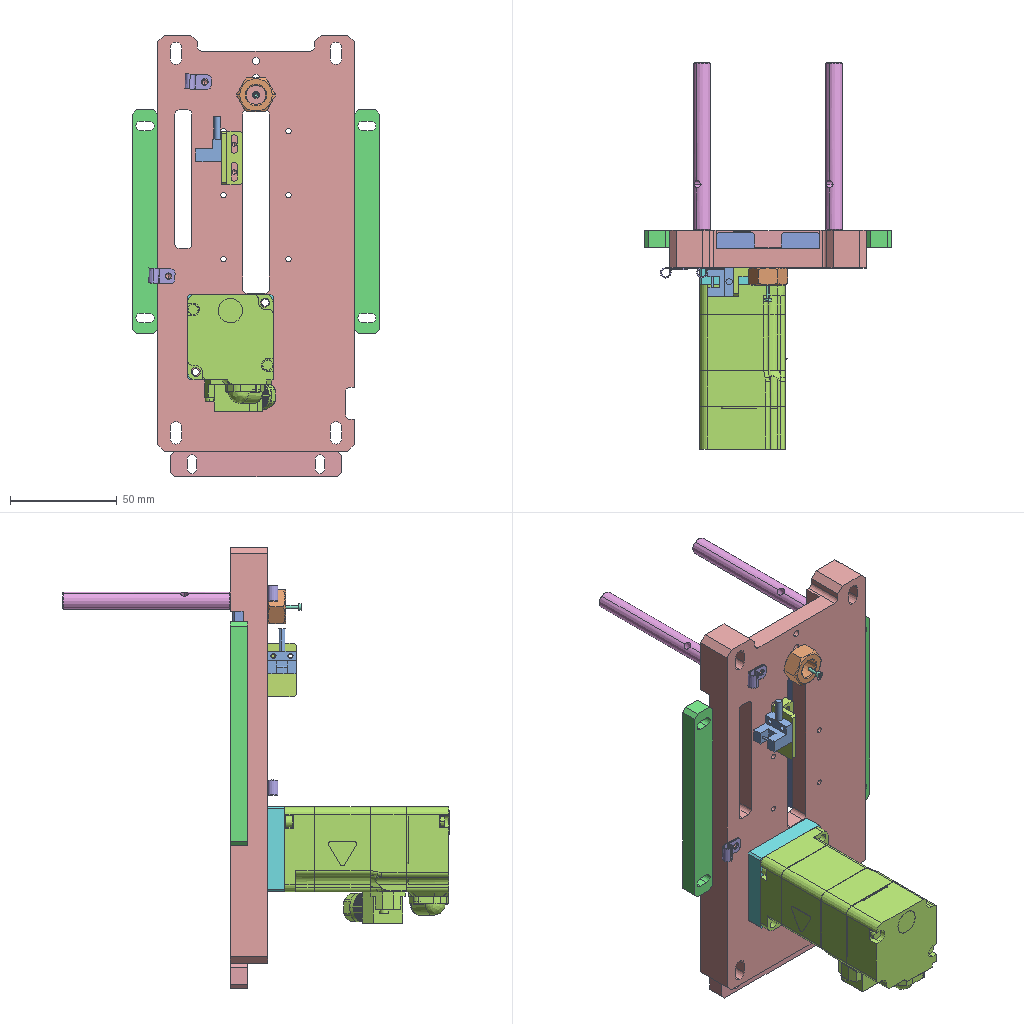Assembly | SolidWorks | 15 different items | 19 placed | box 116 x 181 x 207 mm
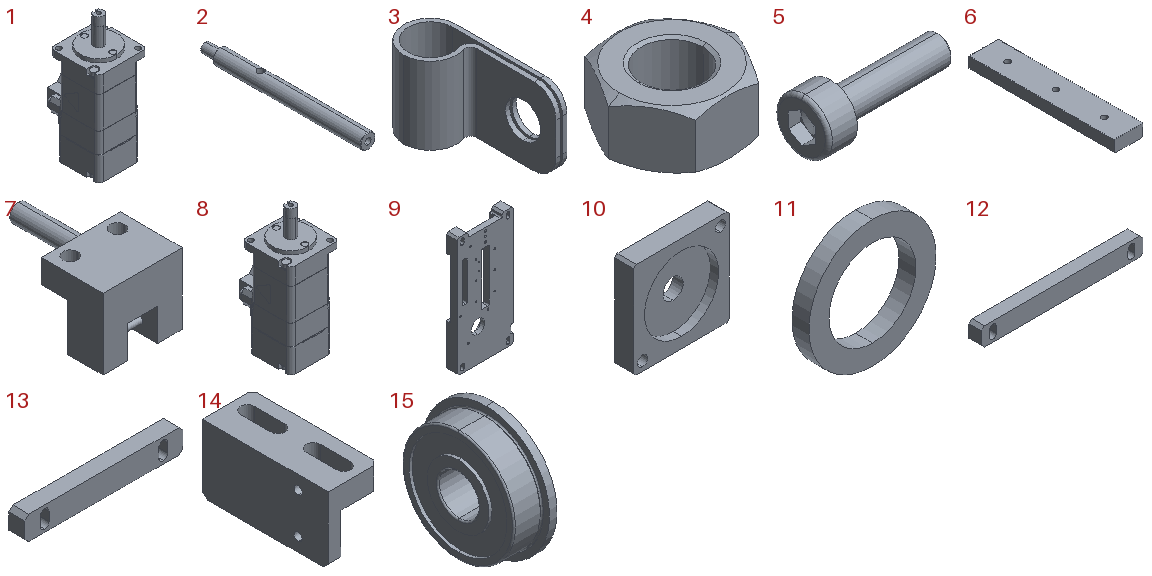Parts list (item | name | quantity | parent item | size | volume | features):
1 | (subassembly) | x1 | - | 41.18 x 54.7 x 102.1 mm | 126795 mm3 | -
2 | - | x2 | - | 8 x 86.5 x 8 mm | 3934 mm3 | features ICE 2, Chamfer 1, Extrusion 1, HoleWzd 1, RevCut 1
3 | - | x2 | - | 4.8 x 12.4 x 7 mm | 75.143 mm3 | features Extrusion 1, Fillet 1, ICE 1
4 | - | x1 | - | 18.475 x 16 x 8.4 mm | 1302 mm3 | features RevCut 2, Chamfer 1, Extrusion 1, LPattern 1
5 | - | x1 | - | 7.6 x 3 x 3 mm | 21.652 mm3 | features Fillet 2, RevCut 2, Boss 1, Chamfer 1, Cut 1, Extrusion 1, LPattern 1
6 | - | x2 | - | 18 x 90 x 7.5 mm | 11592 mm3 | features ICE 2, LPattern 2, Chamfer 1, Extrusion 1
7 | - | x1 | - | 13.4 x 21 x 12 mm | 1080 mm3 | features ICE 4, Extrusion 1
8 | - | x1 | in 1 | 41.18 x 54.7 x 102.1 mm | 126795 mm3 | features BaseBody 15
9 | - | x1 | - | 92 x 17.5 x 195 mm | 172587 mm3 | features ICE 10, HoleWzd 7, Cut 4, Fillet 4, 3DProfileFeature 3, Chamfer 3, Extrusion 1, LPattern 1
10 | - | x1 | - | 40 x 8 x 40 mm | 9655 mm3 | features ICE 2, Chamfer 1, Cut 1, Extrusion 1
11 | - | x1 | - | 12 x 1.6 x 12 mm | 96.459 mm3 | features Extrusion 1
12 | - | x2 | - | 105 x 8 x 12 mm | 9474 mm3 | features ICE 2, Chamfer 1, Extrusion 1
13 | - | x1 | - | 80 x 8 x 12 mm | 7038 mm3 | features ICE 2, Chamfer 1, Extrusion 1
14 | - | x1 | - | 10 x 25 x 13.4 mm | 1439 mm3 | features Chamfer 1, Cut 1, Extrusion 1, HoleWzd 1, ICE 1
15 | - | x1 | - | 7 x 25 x 25 mm | 2247 mm3 | features RefAxis 3, 3DProfileFeature 1, Revolution 1
Mates (type | each side: item.copy, entity, surface, feature):
Coincident | 9.1 face plane Cut-Extrude4 | 6.1 face plane Boss-Extrude1
Coincident | 9.1 face plane Cut-Extrude4 | 6.2 face plane Boss-Extrude1
Concentric | 9.1 face cylinder Cut-Extrude1 | 8.1 face cylinder Input1
Coincident | 9.1 face plane Boss-Extrude1 | 10.1 face plane Boss-Extrude1
Parallel | 9.1 face plane Boss-Extrude1 | 10.1 face plane Boss-Extrude1
Concentric | 8.1 face cylinder Input1 | 10.1 face cylinder Cut-Extrude2
Coincident | 8.1 face plane Input1 | 10.1 face plane Boss-Extrude1 | 2 times
Concentric | 9.1 face cylinder Cut-Extrude1 | 15.1 face cylinder Revolve1
Coincident | 9.1 face plane Cut-Extrude7 | 15.1 face plane Revolve1
Concentric | 8.1 face cylinder Input1 | 11.1 face cylinder Boss-Extrude1
Coincident | 15.1 face plane Revolve1 | 11.1 face plane Boss-Extrude1
Coincident | 9.1 face plane Boss-Extrude1 | 12.1 face plane Boss-Extrude1 | 2 times
Coincident | 12.2 face plane Boss-Extrude1 | 12.1 face plane Boss-Extrude1
Coincident | 9.1 face plane Boss-Extrude1 | 13.1 face plane Boss-Extrude1
Coincident | 9.1 face plane Cut-Extrude5 | 13.1 face plane Boss-Extrude1
DistanceDim | 13.1 face plane Boss-Extrude1 | 9.1 face plane Boss-Extrude1
Parallel | 9.1 face plane Cut-Extrude10 | 7.1 face plane Boss-Extrude1
Coincident | 7.1 face plane Boss-Extrude1 | 14.1 face plane Boss-Extrude1
Coincident | 9.1 face plane Boss-Extrude1 | 14.1 face plane Boss-Extrude1
Coincident | 9.1 face plane Cut-Extrude3 | 14.1 face plane Boss-Extrude1
DistanceDim | 14.1 face plane Boss-Extrude1 | 9.1 face plane Boss-Extrude2
Coincident | 9.1 face plane Boss-Extrude1 | 12.2 face plane Boss-Extrude1 | 2 times
DistanceDim | 12.2 face plane Boss-Extrude1 | 9.1 face plane Boss-Extrude2
Coincident | 9.1 face plane Boss-Extrude1 | 2.1 face plane Boss-Extrude1
Concentric | 9.1 face cylinder M4 Tapped Hole4 | 2.1 face cylinder Boss-Extrude1
Concentric | 9.1 face cylinder M4 Tapped Hole4 | 2.2 face cylinder Boss-Extrude2
Coincident | 9.1 face plane Boss-Extrude1 | 2.2 face plane Boss-Extrude1
Concentric | 9.1 face cylinder M4 Tapped Hole3 | 5.1 face cylinder BaseBody
Concentric | 5.1 face cylinder BaseBody | 4.1 face cone EndChamfer
Coincident | 9.1 face plane Boss-Extrude1 | 4.1 face plane BaseNut
Concentric | 9.1 face cylinder M3 Tapped Hole1 | 6.2 face cylinder LPattern1
Concentric | 9.1 face cylinder M3 Tapped Hole1 | 6.1 face cylinder LPattern1
Concentric | 9.1 face cylinder M3 Tapped Hole1 | 6.2 face cylinder Cut-Extrude2
Concentric | 9.1 face cylinder M3 Tapped Hole1 | 6.1 face cylinder Cut-Extrude2
Concentric | 7.1 face cylinder Cut-Extrude1 | 14.1 face cylinder M2 Tapped Hole1 | 2 times
Coincident | 9.1 face plane Boss-Extrude1 | 3.1 face plane Boss-Extrude1
Concentric | 9.1 face cylinder M3 Tapped Hole2 | 3.1 face cylinder Cut-Extrude1
Coincident | 9.1 face plane Boss-Extrude1 | 3.2 face plane Boss-Extrude1
Concentric | 9.1 face cylinder M3 Tapped Hole3 | 3.2 face cylinder Cut-Extrude1